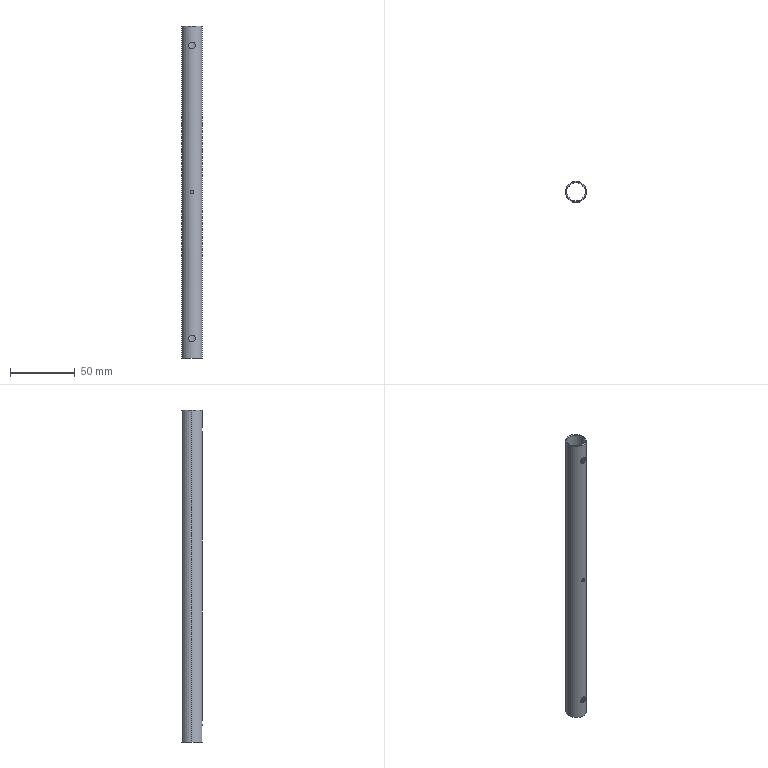Part | SolidWorks | features BaseBody 1 | 1 solid | 12 faces | box 16 x 16 x 256 mm | volume 9739 mm3 | cylinder 10 | plane 2 | commonest cylinder face diameters 5.2 x4 3 x2 14.4 x2 16 x2
STEP:
#1=CARTESIAN_POINT('',(-8.,0.,256.));
#2=VERTEX_POINT('',#1);
#3=CARTESIAN_POINT('',(8.,0.,256.));
#4=VERTEX_POINT('',#3);
#5=CARTESIAN_POINT('',(0.,0.,256.));
#6=DIRECTION('',(0.,0.,-1.));
#7=DIRECTION('',(-1.,0.,0.));
#8=AXIS2_PLACEMENT_3D('',#5,#6,#7);
#9=CIRCLE('',#8,8.);
#10=EDGE_CURVE('',#2,#4,#9,.T.);
#11=ORIENTED_EDGE('',*,*,#10,.T.);
#12=CARTESIAN_POINT('',(8.,0.,0.));
#13=VERTEX_POINT('',#12);
#14=CARTESIAN_POINT('',(8.,0.,256.));
#15=DIRECTION('',(0.,0.,-1.));
#16=VECTOR('',#15,1000.);
#17=LINE('',#14,#16);
#18=EDGE_CURVE('',#4,#13,#17,.T.);
#19=ORIENTED_EDGE('',*,*,#18,.T.);
#20=CARTESIAN_POINT('',(-8.,0.,0.));
#21=VERTEX_POINT('',#20);
#22=CARTESIAN_POINT('',(0.,0.,0.));
#23=DIRECTION('',(0.,0.,1.));
#24=DIRECTION('',(-1.,0.,0.));
#25=AXIS2_PLACEMENT_3D('',#22,#23,#24);
#26=CIRCLE('',#25,8.);
#27=EDGE_CURVE('',#13,#21,#26,.T.);
#28=ORIENTED_EDGE('',*,*,#27,.T.);
#29=CARTESIAN_POINT('',(-8.,0.,256.));
#30=DIRECTION('',(0.,0.,-1.));
#31=VECTOR('',#30,1000.);
#32=LINE('',#29,#31);
#33=EDGE_CURVE('',#2,#21,#32,.T.);
#34=ORIENTED_EDGE('',*,*,#33,.F.);
#35=EDGE_LOOP('',(#11,#19,#28,#34));
#36=FACE_OUTER_BOUND('',#35,.T.);
#37=CARTESIAN_POINT('',(0.,0.,256.));
#38=DIRECTION('',(0.,0.,-1.));
#39=DIRECTION('',(-1.,0.,0.));
#40=AXIS2_PLACEMENT_3D('',#37,#38,#39);
#41=CYLINDRICAL_SURFACE('',#40,8.);
#42=ADVANCED_FACE('',(#36),#41,.T.);
#43=CARTESIAN_POINT('',(0.,-8.,126.5));
#44=VERTEX_POINT('',#43);
#45=CARTESIAN_POINT('',(0.,-8.,129.5));
#46=VERTEX_POINT('',#45);
#47=CARTESIAN_POINT('',(0.,-8.,126.5));
#48=CARTESIAN_POINT('',(-0.09932,-8.,126.5));
#49=CARTESIAN_POINT('',(-0.1969,-7.998,126.51));
#50=CARTESIAN_POINT('',(-0.3889,-7.991,126.548));
#51=CARTESIAN_POINT('',(-0.4843,-7.986,126.577));
#52=CARTESIAN_POINT('',(-0.6658,-7.973,126.652));
#53=CARTESIAN_POINT('',(-0.7519,-7.965,126.698));
#54=CARTESIAN_POINT('',(-0.9148,-7.948,126.807));
#55=CARTESIAN_POINT('',(-0.9917,-7.939,126.87));
#56=CARTESIAN_POINT('',(-1.199,-7.911,127.077));
#57=CARTESIAN_POINT('',(-1.31,-7.892,127.244));
#58=CARTESIAN_POINT('',(-1.46,-7.866,127.605));
#59=CARTESIAN_POINT('',(-1.5,-7.858,127.803));
#60=CARTESIAN_POINT('',(-1.5,-7.858,128.097));
#61=CARTESIAN_POINT('',(-1.49,-7.86,128.196));
#62=CARTESIAN_POINT('',(-1.452,-7.867,128.389));
#63=CARTESIAN_POINT('',(-1.424,-7.872,128.483));
#64=CARTESIAN_POINT('',(-1.311,-7.892,128.755));
#65=CARTESIAN_POINT('',(-1.201,-7.911,128.92));
#66=CARTESIAN_POINT('',(-0.9916,-7.939,129.13));
#67=CARTESIAN_POINT('',(-0.9161,-7.948,129.192));
#68=CARTESIAN_POINT('',(-0.7539,-7.965,129.3));
#69=CARTESIAN_POINT('',(-0.6662,-7.973,129.348));
#70=CARTESIAN_POINT('',(-0.3942,-7.992,129.461));
#71=CARTESIAN_POINT('',(-0.1986,-8.,129.5));
#72=CARTESIAN_POINT('',(0.,-8.,129.5));
#73=B_SPLINE_CURVE_WITH_KNOTS('',3,(#47,#48,#49,#50,#51,#52,#53,#54,#55,#56,#57,#58,#59,#60,#61,#62,#63,#64,#65,#66,#67,#68,#69,#70,#71,#72),.UNSPECIFIED.,.F.,.F.,(4,2,2,2,2,2,2,2,2,2,2,2,4),(0.,0.0002937,0.0005874,0.000881,0.001175,0.001762,0.002349,0.002643,0.002937,0.003524,0.003818,0.004112,0.004699),.UNSPECIFIED.);
#74=EDGE_CURVE('',#44,#46,#73,.T.);
#75=ORIENTED_EDGE('',*,*,#74,.F.);
#76=CARTESIAN_POINT('',(0.,-7.2,126.5));
#77=VERTEX_POINT('',#76);
#78=CARTESIAN_POINT('',(0.,-8.,126.5));
#79=DIRECTION('',(0.,1.,0.));
#80=VECTOR('',#79,1000.);
#81=LINE('',#78,#80);
#82=EDGE_CURVE('',#44,#77,#81,.T.);
#83=ORIENTED_EDGE('',*,*,#82,.T.);
#84=CARTESIAN_POINT('',(0.,-7.2,129.5));
#85=VERTEX_POINT('',#84);
#86=CARTESIAN_POINT('',(0.,-7.2,129.5));
#87=CARTESIAN_POINT('',(-0.09937,-7.2,129.5));
#88=CARTESIAN_POINT('',(-0.197,-7.198,129.49));
#89=CARTESIAN_POINT('',(-0.3891,-7.19,129.452));
#90=CARTESIAN_POINT('',(-0.4845,-7.184,129.423));
#91=CARTESIAN_POINT('',(-0.666,-7.17,129.348));
#92=CARTESIAN_POINT('',(-0.752,-7.161,129.302));
#93=CARTESIAN_POINT('',(-0.9149,-7.142,129.193));
#94=CARTESIAN_POINT('',(-0.9917,-7.132,129.13));
#95=CARTESIAN_POINT('',(-1.199,-7.101,128.923));
#96=CARTESIAN_POINT('',(-1.31,-7.08,128.756));
#97=CARTESIAN_POINT('',(-1.46,-7.051,128.395));
#98=CARTESIAN_POINT('',(-1.5,-7.042,128.197));
#99=CARTESIAN_POINT('',(-1.5,-7.042,127.903));
#100=CARTESIAN_POINT('',(-1.49,-7.044,127.803));
#101=CARTESIAN_POINT('',(-1.452,-7.052,127.611));
#102=CARTESIAN_POINT('',(-1.424,-7.058,127.517));
#103=CARTESIAN_POINT('',(-1.311,-7.08,127.244));
#104=CARTESIAN_POINT('',(-1.2,-7.101,127.079));
#105=CARTESIAN_POINT('',(-0.9916,-7.132,126.87));
#106=CARTESIAN_POINT('',(-0.9162,-7.142,126.808));
#107=CARTESIAN_POINT('',(-0.7541,-7.161,126.7));
#108=CARTESIAN_POINT('',(-0.6663,-7.17,126.653));
#109=CARTESIAN_POINT('',(-0.3945,-7.191,126.54));
#110=CARTESIAN_POINT('',(-0.1988,-7.2,126.5));
#111=CARTESIAN_POINT('',(0.,-7.2,126.5));
#112=B_SPLINE_CURVE_WITH_KNOTS('',3,(#86,#87,#88,#89,#90,#91,#92,#93,#94,#95,#96,#97,#98,#99,#100,#101,#102,#103,#104,#105,#106,#107,#108,#109,#110,#111),.UNSPECIFIED.,.F.,.F.,(4,2,2,2,2,2,2,2,2,2,2,2,4),(0.,0.0002938,0.0005877,0.0008815,0.001175,0.001763,0.002351,0.002644,0.002938,0.003526,0.00382,0.004114,0.004701),.UNSPECIFIED.);
#113=EDGE_CURVE('',#85,#77,#112,.T.);
#114=ORIENTED_EDGE('',*,*,#113,.F.);
#115=CARTESIAN_POINT('',(0.,-8.,129.5));
#116=DIRECTION('',(0.,1.,0.));
#117=VECTOR('',#116,1000.);
#118=LINE('',#115,#117);
#119=EDGE_CURVE('',#46,#85,#118,.T.);
#120=ORIENTED_EDGE('',*,*,#119,.F.);
#121=EDGE_LOOP('',(#75,#83,#114,#120));
#122=FACE_OUTER_BOUND('',#121,.T.);
#123=CARTESIAN_POINT('',(0.,-8.,128.));
#124=DIRECTION('',(0.,1.,0.));
#125=DIRECTION('',(0.,0.,1.));
#126=AXIS2_PLACEMENT_3D('',#123,#124,#125);
#127=CYLINDRICAL_SURFACE('',#126,1.5);
#128=ADVANCED_FACE('',(#122),#127,.F.);
#129=CARTESIAN_POINT('',(0.,-8.,238.4));
#130=VERTEX_POINT('',#129);
#131=CARTESIAN_POINT('',(0.,-8.,243.6));
#132=VERTEX_POINT('',#131);
#133=CARTESIAN_POINT('',(0.,-8.,238.4));
#134=CARTESIAN_POINT('',(-0.173,-8.,238.4));
#135=CARTESIAN_POINT('',(-0.3429,-7.994,238.417));
#136=CARTESIAN_POINT('',(-0.6767,-7.973,238.484));
#137=CARTESIAN_POINT('',(-0.8425,-7.957,238.534));
#138=CARTESIAN_POINT('',(-1.157,-7.918,238.665));
#139=CARTESIAN_POINT('',(-1.306,-7.894,238.745));
#140=CARTESIAN_POINT('',(-1.587,-7.842,238.934));
#141=CARTESIAN_POINT('',(-1.72,-7.814,239.043));
#142=CARTESIAN_POINT('',(-2.077,-7.73,239.4));
#143=CARTESIAN_POINT('',(-2.27,-7.672,239.688));
#144=CARTESIAN_POINT('',(-2.465,-7.611,240.156));
#145=CARTESIAN_POINT('',(-2.516,-7.594,240.321));
#146=CARTESIAN_POINT('',(-2.583,-7.572,240.657));
#147=CARTESIAN_POINT('',(-2.6,-7.566,240.826));
#148=CARTESIAN_POINT('',(-2.6,-7.566,241.168));
#149=CARTESIAN_POINT('',(-2.583,-7.572,241.342));
#150=CARTESIAN_POINT('',(-2.516,-7.594,241.676));
#151=CARTESIAN_POINT('',(-2.467,-7.61,241.839));
#152=CARTESIAN_POINT('',(-2.336,-7.652,242.155));
#153=CARTESIAN_POINT('',(-2.255,-7.676,242.305));
#154=CARTESIAN_POINT('',(-2.068,-7.729,242.585));
#155=CARTESIAN_POINT('',(-1.959,-7.757,242.718));
#156=CARTESIAN_POINT('',(-1.72,-7.814,242.957));
#157=CARTESIAN_POINT('',(-1.59,-7.842,243.064));
#158=CARTESIAN_POINT('',(-1.309,-7.893,243.253));
#159=CARTESIAN_POINT('',(-1.157,-7.917,243.334));
#160=CARTESIAN_POINT('',(-0.8442,-7.957,243.465));
#161=CARTESIAN_POINT('',(-0.682,-7.973,243.515));
#162=CARTESIAN_POINT('',(-0.3459,-7.994,243.583));
#163=CARTESIAN_POINT('',(-0.173,-8.,243.6));
#164=CARTESIAN_POINT('',(0.,-8.,243.6));
#165=B_SPLINE_CURVE_WITH_KNOTS('',3,(#133,#134,#135,#136,#137,#138,#139,#140,#141,#142,#143,#144,#145,#146,#147,#148,#149,#150,#151,#152,#153,#154,#155,#156,#157,#158,#159,#160,#161,#162,#163,#164),.UNSPECIFIED.,.F.,.F.,(4,2,2,2,2,2,2,2,2,2,2,2,2,2,2,4),(0.,0.0005114,0.001023,0.001534,0.002045,0.003068,0.003579,0.004091,0.004602,0.005114,0.005625,0.006136,0.006648,0.007159,0.00767,0.008182),.UNSPECIFIED.);
#166=EDGE_CURVE('',#130,#132,#165,.T.);
#167=ORIENTED_EDGE('',*,*,#166,.F.);
#168=CARTESIAN_POINT('',(0.,-7.2,238.4));
#169=VERTEX_POINT('',#168);
#170=CARTESIAN_POINT('',(0.,-8.,238.4));
#171=DIRECTION('',(0.,1.,0.));
#172=VECTOR('',#171,1000.);
#173=LINE('',#170,#172);
#174=EDGE_CURVE('',#130,#169,#173,.T.);
#175=ORIENTED_EDGE('',*,*,#174,.T.);
#176=CARTESIAN_POINT('',(0.,-7.2,243.6));
#177=VERTEX_POINT('',#176);
#178=CARTESIAN_POINT('',(0.,-7.2,243.6));
#179=CARTESIAN_POINT('',(-0.1733,-7.2,243.6));
#180=CARTESIAN_POINT('',(-0.3434,-7.194,243.583));
#181=CARTESIAN_POINT('',(-0.6777,-7.17,243.516));
#182=CARTESIAN_POINT('',(-0.8436,-7.152,243.465));
#183=CARTESIAN_POINT('',(-1.158,-7.108,243.334));
#184=CARTESIAN_POINT('',(-1.307,-7.082,243.254));
#185=CARTESIAN_POINT('',(-1.588,-7.024,243.066));
#186=CARTESIAN_POINT('',(-1.72,-6.993,242.957));
#187=CARTESIAN_POINT('',(-2.076,-6.898,242.6));
#188=CARTESIAN_POINT('',(-2.269,-6.834,242.313));
#189=CARTESIAN_POINT('',(-2.465,-6.765,241.845));
#190=CARTESIAN_POINT('',(-2.515,-6.746,241.68));
#191=CARTESIAN_POINT('',(-2.583,-6.721,241.344));
#192=CARTESIAN_POINT('',(-2.6,-6.714,241.174));
#193=CARTESIAN_POINT('',(-2.6,-6.714,240.832));
#194=CARTESIAN_POINT('',(-2.583,-6.721,240.658));
#195=CARTESIAN_POINT('',(-2.516,-6.746,240.323));
#196=CARTESIAN_POINT('',(-2.467,-6.765,240.161));
#197=CARTESIAN_POINT('',(-2.335,-6.811,239.844));
#198=CARTESIAN_POINT('',(-2.255,-6.839,239.694));
#199=CARTESIAN_POINT('',(-2.067,-6.898,239.414));
#200=CARTESIAN_POINT('',(-1.959,-6.93,239.282));
#201=CARTESIAN_POINT('',(-1.72,-6.993,239.043));
#202=CARTESIAN_POINT('',(-1.591,-7.024,238.936));
#203=CARTESIAN_POINT('',(-1.31,-7.081,238.748));
#204=CARTESIAN_POINT('',(-1.158,-7.108,238.666));
#205=CARTESIAN_POINT('',(-0.8456,-7.152,238.536));
#206=CARTESIAN_POINT('',(-0.6833,-7.169,238.486));
#207=CARTESIAN_POINT('',(-0.3462,-7.194,238.417));
#208=CARTESIAN_POINT('',(-0.1733,-7.2,238.4));
#209=CARTESIAN_POINT('',(0.,-7.2,238.4));
#210=B_SPLINE_CURVE_WITH_KNOTS('',3,(#178,#179,#180,#181,#182,#183,#184,#185,#186,#187,#188,#189,#190,#191,#192,#193,#194,#195,#196,#197,#198,#199,#200,#201,#202,#203,#204,#205,#206,#207,#208,#209),.UNSPECIFIED.,.F.,.F.,(4,2,2,2,2,2,2,2,2,2,2,2,2,2,2,4),(0.,0.0005122,0.001024,0.001537,0.002049,0.003073,0.003585,0.004098,0.00461,0.005122,0.005634,0.006146,0.006659,0.007171,0.007683,0.008195),.UNSPECIFIED.);
#211=EDGE_CURVE('',#177,#169,#210,.T.);
#212=ORIENTED_EDGE('',*,*,#211,.F.);
#213=CARTESIAN_POINT('',(0.,-8.,243.6));
#214=DIRECTION('',(0.,1.,0.));
#215=VECTOR('',#214,1000.);
#216=LINE('',#213,#215);
#217=EDGE_CURVE('',#132,#177,#216,.T.);
#218=ORIENTED_EDGE('',*,*,#217,.F.);
#219=EDGE_LOOP('',(#167,#175,#212,#218));
#220=FACE_OUTER_BOUND('',#219,.T.);
#221=CARTESIAN_POINT('',(0.,-8.,241.));
#222=DIRECTION('',(0.,1.,0.));
#223=DIRECTION('',(0.,0.,1.));
#224=AXIS2_PLACEMENT_3D('',#221,#222,#223);
#225=CYLINDRICAL_SURFACE('',#224,2.6);
#226=ADVANCED_FACE('',(#220),#225,.F.);
#227=CARTESIAN_POINT('',(0.,-8.,12.4));
#228=VERTEX_POINT('',#227);
#229=CARTESIAN_POINT('',(0.,-8.,17.6));
#230=VERTEX_POINT('',#229);
#231=CARTESIAN_POINT('',(0.,-8.,12.4));
#232=CARTESIAN_POINT('',(-0.173,-8.,12.4));
#233=CARTESIAN_POINT('',(-0.3429,-7.994,12.417));
#234=CARTESIAN_POINT('',(-0.6767,-7.973,12.484));
#235=CARTESIAN_POINT('',(-0.8425,-7.957,12.534));
#236=CARTESIAN_POINT('',(-1.157,-7.918,12.665));
#237=CARTESIAN_POINT('',(-1.306,-7.894,12.745));
#238=CARTESIAN_POINT('',(-1.587,-7.842,12.934));
#239=CARTESIAN_POINT('',(-1.72,-7.814,13.043));
#240=CARTESIAN_POINT('',(-2.077,-7.73,13.4));
#241=CARTESIAN_POINT('',(-2.27,-7.672,13.688));
#242=CARTESIAN_POINT('',(-2.465,-7.611,14.156));
#243=CARTESIAN_POINT('',(-2.516,-7.594,14.321));
#244=CARTESIAN_POINT('',(-2.583,-7.572,14.657));
#245=CARTESIAN_POINT('',(-2.6,-7.566,14.826));
#246=CARTESIAN_POINT('',(-2.6,-7.566,15.168));
#247=CARTESIAN_POINT('',(-2.583,-7.572,15.342));
#248=CARTESIAN_POINT('',(-2.516,-7.594,15.676));
#249=CARTESIAN_POINT('',(-2.467,-7.61,15.839));
#250=CARTESIAN_POINT('',(-2.336,-7.652,16.155));
#251=CARTESIAN_POINT('',(-2.255,-7.676,16.305));
#252=CARTESIAN_POINT('',(-2.068,-7.729,16.585));
#253=CARTESIAN_POINT('',(-1.959,-7.757,16.718));
#254=CARTESIAN_POINT('',(-1.72,-7.814,16.957));
#255=CARTESIAN_POINT('',(-1.59,-7.842,17.064));
#256=CARTESIAN_POINT('',(-1.309,-7.893,17.253));
#257=CARTESIAN_POINT('',(-1.157,-7.917,17.334));
#258=CARTESIAN_POINT('',(-0.8442,-7.957,17.465));
#259=CARTESIAN_POINT('',(-0.682,-7.973,17.515));
#260=CARTESIAN_POINT('',(-0.3459,-7.994,17.583));
#261=CARTESIAN_POINT('',(-0.173,-8.,17.6));
#262=CARTESIAN_POINT('',(0.,-8.,17.6));
#263=B_SPLINE_CURVE_WITH_KNOTS('',3,(#231,#232,#233,#234,#235,#236,#237,#238,#239,#240,#241,#242,#243,#244,#245,#246,#247,#248,#249,#250,#251,#252,#253,#254,#255,#256,#257,#258,#259,#260,#261,#262),.UNSPECIFIED.,.F.,.F.,(4,2,2,2,2,2,2,2,2,2,2,2,2,2,2,4),(0.,0.0005114,0.001023,0.001534,0.002045,0.003068,0.003579,0.004091,0.004602,0.005114,0.005625,0.006136,0.006648,0.007159,0.00767,0.008182),.UNSPECIFIED.);
#264=EDGE_CURVE('',#228,#230,#263,.T.);
#265=ORIENTED_EDGE('',*,*,#264,.F.);
#266=CARTESIAN_POINT('',(0.,-7.2,12.4));
#267=VERTEX_POINT('',#266);
#268=CARTESIAN_POINT('',(0.,-8.,12.4));
#269=DIRECTION('',(0.,1.,0.));
#270=VECTOR('',#269,1000.);
#271=LINE('',#268,#270);
#272=EDGE_CURVE('',#228,#267,#271,.T.);
#273=ORIENTED_EDGE('',*,*,#272,.T.);
#274=CARTESIAN_POINT('',(0.,-7.2,17.6));
#275=VERTEX_POINT('',#274);
#276=CARTESIAN_POINT('',(0.,-7.2,17.6));
#277=CARTESIAN_POINT('',(-0.1733,-7.2,17.6));
#278=CARTESIAN_POINT('',(-0.3434,-7.194,17.583));
#279=CARTESIAN_POINT('',(-0.6777,-7.17,17.516));
#280=CARTESIAN_POINT('',(-0.8436,-7.152,17.465));
#281=CARTESIAN_POINT('',(-1.158,-7.108,17.334));
#282=CARTESIAN_POINT('',(-1.307,-7.082,17.254));
#283=CARTESIAN_POINT('',(-1.588,-7.024,17.066));
#284=CARTESIAN_POINT('',(-1.72,-6.993,16.957));
#285=CARTESIAN_POINT('',(-2.076,-6.898,16.6));
#286=CARTESIAN_POINT('',(-2.269,-6.834,16.313));
#287=CARTESIAN_POINT('',(-2.465,-6.765,15.845));
#288=CARTESIAN_POINT('',(-2.515,-6.746,15.68));
#289=CARTESIAN_POINT('',(-2.583,-6.721,15.344));
#290=CARTESIAN_POINT('',(-2.6,-6.714,15.174));
#291=CARTESIAN_POINT('',(-2.6,-6.714,14.832));
#292=CARTESIAN_POINT('',(-2.583,-6.721,14.658));
#293=CARTESIAN_POINT('',(-2.516,-6.746,14.323));
#294=CARTESIAN_POINT('',(-2.467,-6.765,14.161));
#295=CARTESIAN_POINT('',(-2.335,-6.811,13.844));
#296=CARTESIAN_POINT('',(-2.255,-6.839,13.694));
#297=CARTESIAN_POINT('',(-2.067,-6.898,13.414));
#298=CARTESIAN_POINT('',(-1.959,-6.93,13.282));
#299=CARTESIAN_POINT('',(-1.72,-6.993,13.043));
#300=CARTESIAN_POINT('',(-1.591,-7.024,12.936));
#301=CARTESIAN_POINT('',(-1.31,-7.081,12.748));
#302=CARTESIAN_POINT('',(-1.158,-7.108,12.666));
#303=CARTESIAN_POINT('',(-0.8456,-7.152,12.536));
#304=CARTESIAN_POINT('',(-0.6833,-7.169,12.486));
#305=CARTESIAN_POINT('',(-0.3462,-7.194,12.417));
#306=CARTESIAN_POINT('',(-0.1733,-7.2,12.4));
#307=CARTESIAN_POINT('',(0.,-7.2,12.4));
#308=B_SPLINE_CURVE_WITH_KNOTS('',3,(#276,#277,#278,#279,#280,#281,#282,#283,#284,#285,#286,#287,#288,#289,#290,#291,#292,#293,#294,#295,#296,#297,#298,#299,#300,#301,#302,#303,#304,#305,#306,#307),.UNSPECIFIED.,.F.,.F.,(4,2,2,2,2,2,2,2,2,2,2,2,2,2,2,4),(0.,0.0005122,0.001024,0.001537,0.002049,0.003073,0.003585,0.004098,0.00461,0.005122,0.005634,0.006146,0.006659,0.007171,0.007683,0.008195),.UNSPECIFIED.);
#309=EDGE_CURVE('',#275,#267,#308,.T.);
#310=ORIENTED_EDGE('',*,*,#309,.F.);
#311=CARTESIAN_POINT('',(0.,-8.,17.6));
#312=DIRECTION('',(0.,1.,0.));
#313=VECTOR('',#312,1000.);
#314=LINE('',#311,#313);
#315=EDGE_CURVE('',#230,#275,#314,.T.);
#316=ORIENTED_EDGE('',*,*,#315,.F.);
#317=EDGE_LOOP('',(#265,#273,#310,#316));
#318=FACE_OUTER_BOUND('',#317,.T.);
#319=CARTESIAN_POINT('',(0.,-8.,15.));
#320=DIRECTION('',(0.,1.,0.));
#321=DIRECTION('',(0.,0.,1.));
#322=AXIS2_PLACEMENT_3D('',#319,#320,#321);
#323=CYLINDRICAL_SURFACE('',#322,2.6);
#324=ADVANCED_FACE('',(#318),#323,.F.);
#325=ORIENTED_EDGE('',*,*,#113,.T.);
#326=CARTESIAN_POINT('',(0.,-7.2,126.5));
#327=CARTESIAN_POINT('',(0.09937,-7.2,126.5));
#328=CARTESIAN_POINT('',(0.197,-7.198,126.51));
#329=CARTESIAN_POINT('',(0.3891,-7.19,126.548));
#330=CARTESIAN_POINT('',(0.4845,-7.184,126.577));
#331=CARTESIAN_POINT('',(0.666,-7.17,126.652));
#332=CARTESIAN_POINT('',(0.752,-7.161,126.698));
#333=CARTESIAN_POINT('',(0.9149,-7.142,126.807));
#334=CARTESIAN_POINT('',(0.9917,-7.132,126.87));
#335=CARTESIAN_POINT('',(1.199,-7.101,127.077));
#336=CARTESIAN_POINT('',(1.31,-7.08,127.244));
#337=CARTESIAN_POINT('',(1.46,-7.051,127.605));
#338=CARTESIAN_POINT('',(1.5,-7.042,127.803));
#339=CARTESIAN_POINT('',(1.5,-7.042,128.097));
#340=CARTESIAN_POINT('',(1.49,-7.044,128.197));
#341=CARTESIAN_POINT('',(1.452,-7.052,128.389));
#342=CARTESIAN_POINT('',(1.424,-7.058,128.483));
#343=CARTESIAN_POINT('',(1.311,-7.08,128.756));
#344=CARTESIAN_POINT('',(1.2,-7.101,128.921));
#345=CARTESIAN_POINT('',(0.9916,-7.132,129.13));
#346=CARTESIAN_POINT('',(0.9162,-7.142,129.192));
#347=CARTESIAN_POINT('',(0.7541,-7.161,129.3));
#348=CARTESIAN_POINT('',(0.6663,-7.17,129.347));
#349=CARTESIAN_POINT('',(0.3945,-7.191,129.46));
#350=CARTESIAN_POINT('',(0.1987,-7.2,129.5));
#351=CARTESIAN_POINT('',(0.,-7.2,129.5));
#352=B_SPLINE_CURVE_WITH_KNOTS('',3,(#326,#327,#328,#329,#330,#331,#332,#333,#334,#335,#336,#337,#338,#339,#340,#341,#342,#343,#344,#345,#346,#347,#348,#349,#350,#351),.UNSPECIFIED.,.F.,.F.,(4,2,2,2,2,2,2,2,2,2,2,2,4),(0.004701,0.004995,0.005289,0.005583,0.005877,0.006464,0.007052,0.007346,0.00764,0.008227,0.008521,0.008815,0.009403),.UNSPECIFIED.);
#353=EDGE_CURVE('',#77,#85,#352,.T.);
#354=ORIENTED_EDGE('',*,*,#353,.T.);
#355=EDGE_LOOP('',(#325,#354));
#356=FACE_BOUND('',#355,.T.);
#357=ORIENTED_EDGE('',*,*,#211,.T.);
#358=CARTESIAN_POINT('',(0.,-7.2,238.4));
#359=CARTESIAN_POINT('',(0.1733,-7.2,238.4));
#360=CARTESIAN_POINT('',(0.3434,-7.194,238.417));
#361=CARTESIAN_POINT('',(0.6777,-7.17,238.484));
#362=CARTESIAN_POINT('',(0.8436,-7.152,238.535));
#363=CARTESIAN_POINT('',(1.158,-7.108,238.666));
#364=CARTESIAN_POINT('',(1.307,-7.082,238.746));
#365=CARTESIAN_POINT('',(1.588,-7.024,238.934));
#366=CARTESIAN_POINT('',(1.72,-6.993,239.043));
#367=CARTESIAN_POINT('',(2.076,-6.898,239.4));
#368=CARTESIAN_POINT('',(2.269,-6.834,239.687));
#369=CARTESIAN_POINT('',(2.465,-6.765,240.155));
#370=CARTESIAN_POINT('',(2.515,-6.746,240.32));
#371=CARTESIAN_POINT('',(2.583,-6.721,240.656));
#372=CARTESIAN_POINT('',(2.6,-6.714,240.826));
#373=CARTESIAN_POINT('',(2.6,-6.714,241.168));
#374=CARTESIAN_POINT('',(2.583,-6.721,241.342));
#375=CARTESIAN_POINT('',(2.516,-6.746,241.677));
#376=CARTESIAN_POINT('',(2.467,-6.765,241.839));
#377=CARTESIAN_POINT('',(2.335,-6.811,242.156));
#378=CARTESIAN_POINT('',(2.255,-6.839,242.306));
#379=CARTESIAN_POINT('',(2.067,-6.898,242.586));
#380=CARTESIAN_POINT('',(1.959,-6.93,242.718));
#381=CARTESIAN_POINT('',(1.72,-6.993,242.957));
#382=CARTESIAN_POINT('',(1.591,-7.024,243.064));
#383=CARTESIAN_POINT('',(1.31,-7.081,243.252));
#384=CARTESIAN_POINT('',(1.158,-7.108,243.334));
#385=CARTESIAN_POINT('',(0.8456,-7.152,243.464));
#386=CARTESIAN_POINT('',(0.6833,-7.169,243.514));
#387=CARTESIAN_POINT('',(0.3462,-7.194,243.583));
#388=CARTESIAN_POINT('',(0.1733,-7.2,243.6));
#389=CARTESIAN_POINT('',(0.,-7.2,243.6));
#390=B_SPLINE_CURVE_WITH_KNOTS('',3,(#358,#359,#360,#361,#362,#363,#364,#365,#366,#367,#368,#369,#370,#371,#372,#373,#374,#375,#376,#377,#378,#379,#380,#381,#382,#383,#384,#385,#386,#387,#388,#389),.UNSPECIFIED.,.F.,.F.,(4,2,2,2,2,2,2,2,2,2,2,2,2,2,2,4),(0.008195,0.008707,0.00922,0.009732,0.01024,0.01127,0.01178,0.01229,0.0128,0.01332,0.01383,0.01434,0.01485,0.01536,0.01588,0.01639),.UNSPECIFIED.);
#391=EDGE_CURVE('',#169,#177,#390,.T.);
#392=ORIENTED_EDGE('',*,*,#391,.T.);
#393=EDGE_LOOP('',(#357,#392));
#394=FACE_BOUND('',#393,.T.);
#395=ORIENTED_EDGE('',*,*,#309,.T.);
#396=CARTESIAN_POINT('',(0.,-7.2,12.4));
#397=CARTESIAN_POINT('',(0.1733,-7.2,12.4));
#398=CARTESIAN_POINT('',(0.3434,-7.194,12.417));
#399=CARTESIAN_POINT('',(0.6777,-7.17,12.484));
#400=CARTESIAN_POINT('',(0.8436,-7.152,12.535));
#401=CARTESIAN_POINT('',(1.158,-7.108,12.666));
#402=CARTESIAN_POINT('',(1.307,-7.082,12.746));
#403=CARTESIAN_POINT('',(1.588,-7.024,12.934));
#404=CARTESIAN_POINT('',(1.72,-6.993,13.043));
#405=CARTESIAN_POINT('',(2.076,-6.898,13.4));
#406=CARTESIAN_POINT('',(2.269,-6.834,13.687));
#407=CARTESIAN_POINT('',(2.465,-6.765,14.155));
#408=CARTESIAN_POINT('',(2.515,-6.746,14.32));
#409=CARTESIAN_POINT('',(2.583,-6.721,14.656));
#410=CARTESIAN_POINT('',(2.6,-6.714,14.826));
#411=CARTESIAN_POINT('',(2.6,-6.714,15.168));
#412=CARTESIAN_POINT('',(2.583,-6.721,15.342));
#413=CARTESIAN_POINT('',(2.516,-6.746,15.677));
#414=CARTESIAN_POINT('',(2.467,-6.765,15.839));
#415=CARTESIAN_POINT('',(2.335,-6.811,16.156));
#416=CARTESIAN_POINT('',(2.255,-6.839,16.306));
#417=CARTESIAN_POINT('',(2.067,-6.898,16.586));
#418=CARTESIAN_POINT('',(1.959,-6.93,16.718));
#419=CARTESIAN_POINT('',(1.72,-6.993,16.957));
#420=CARTESIAN_POINT('',(1.591,-7.024,17.064));
#421=CARTESIAN_POINT('',(1.31,-7.081,17.252));
#422=CARTESIAN_POINT('',(1.158,-7.108,17.334));
#423=CARTESIAN_POINT('',(0.8456,-7.152,17.464));
#424=CARTESIAN_POINT('',(0.6833,-7.169,17.514));
#425=CARTESIAN_POINT('',(0.3462,-7.194,17.583));
#426=CARTESIAN_POINT('',(0.1733,-7.2,17.6));
#427=CARTESIAN_POINT('',(0.,-7.2,17.6));
#428=B_SPLINE_CURVE_WITH_KNOTS('',3,(#396,#397,#398,#399,#400,#401,#402,#403,#404,#405,#406,#407,#408,#409,#410,#411,#412,#413,#414,#415,#416,#417,#418,#419,#420,#421,#422,#423,#424,#425,#426,#427),.UNSPECIFIED.,.F.,.F.,(4,2,2,2,2,2,2,2,2,2,2,2,2,2,2,4),(0.008195,0.008707,0.00922,0.009732,0.01024,0.01127,0.01178,0.01229,0.0128,0.01332,0.01383,0.01434,0.01485,0.01536,0.01588,0.01639),.UNSPECIFIED.);
#429=EDGE_CURVE('',#267,#275,#428,.T.);
#430=ORIENTED_EDGE('',*,*,#429,.T.);
#431=EDGE_LOOP('',(#395,#430));
#432=FACE_BOUND('',#431,.T.);
#433=CARTESIAN_POINT('',(7.2,0.,256.));
#434=VERTEX_POINT('',#433);
#435=CARTESIAN_POINT('',(-7.2,0.,256.));
#436=VERTEX_POINT('',#435);
#437=CARTESIAN_POINT('',(0.,0.,256.));
#438=DIRECTION('',(0.,0.,-1.));
#439=DIRECTION('',(-1.,0.,0.));
#440=AXIS2_PLACEMENT_3D('',#437,#438,#439);
#441=CIRCLE('',#440,7.2);
#442=EDGE_CURVE('',#434,#436,#441,.T.);
#443=ORIENTED_EDGE('',*,*,#442,.F.);
#444=CARTESIAN_POINT('',(7.2,0.,0.));
#445=VERTEX_POINT('',#444);
#446=CARTESIAN_POINT('',(7.2,0.,256.));
#447=DIRECTION('',(0.,0.,-1.));
#448=VECTOR('',#447,1000.);
#449=LINE('',#446,#448);
#450=EDGE_CURVE('',#434,#445,#449,.T.);
#451=ORIENTED_EDGE('',*,*,#450,.T.);
#452=CARTESIAN_POINT('',(-7.2,0.,0.));
#453=VERTEX_POINT('',#452);
#454=CARTESIAN_POINT('',(0.,0.,0.));
#455=DIRECTION('',(0.,0.,-1.));
#456=DIRECTION('',(-1.,0.,0.));
#457=AXIS2_PLACEMENT_3D('',#454,#455,#456);
#458=CIRCLE('',#457,7.2);
#459=EDGE_CURVE('',#445,#453,#458,.T.);
#460=ORIENTED_EDGE('',*,*,#459,.T.);
#461=CARTESIAN_POINT('',(-7.2,0.,256.));
#462=DIRECTION('',(0.,0.,-1.));
#463=VECTOR('',#462,1000.);
#464=LINE('',#461,#463);
#465=EDGE_CURVE('',#436,#453,#464,.T.);
#466=ORIENTED_EDGE('',*,*,#465,.F.);
#467=EDGE_LOOP('',(#443,#451,#460,#466));
#468=FACE_OUTER_BOUND('',#467,.T.);
#469=CARTESIAN_POINT('',(0.,0.,256.));
#470=DIRECTION('',(0.,0.,-1.));
#471=DIRECTION('',(-1.,0.,0.));
#472=AXIS2_PLACEMENT_3D('',#469,#470,#471);
#473=CYLINDRICAL_SURFACE('',#472,7.2);
#474=ADVANCED_FACE('',(#356,#394,#432,#468),#473,.F.);
#475=ORIENTED_EDGE('',*,*,#18,.F.);
#476=CARTESIAN_POINT('',(0.,0.,256.));
#477=DIRECTION('',(0.,0.,-1.));
#478=DIRECTION('',(-1.,0.,0.));
#479=AXIS2_PLACEMENT_3D('',#476,#477,#478);
#480=CIRCLE('',#479,8.);
#481=EDGE_CURVE('',#4,#2,#480,.T.);
#482=ORIENTED_EDGE('',*,*,#481,.T.);
#483=ORIENTED_EDGE('',*,*,#33,.T.);
#484=CARTESIAN_POINT('',(0.,0.,0.));
#485=DIRECTION('',(0.,0.,1.));
#486=DIRECTION('',(-1.,0.,0.));
#487=AXIS2_PLACEMENT_3D('',#484,#485,#486);
#488=CIRCLE('',#487,8.);
#489=EDGE_CURVE('',#21,#13,#488,.T.);
#490=ORIENTED_EDGE('',*,*,#489,.T.);
#491=EDGE_LOOP('',(#475,#482,#483,#490));
#492=FACE_OUTER_BOUND('',#491,.T.);
#493=CARTESIAN_POINT('',(0.,-8.,129.5));
#494=CARTESIAN_POINT('',(0.09932,-8.,129.5));
#495=CARTESIAN_POINT('',(0.1969,-7.998,129.49));
#496=CARTESIAN_POINT('',(0.3889,-7.991,129.452));
#497=CARTESIAN_POINT('',(0.4843,-7.986,129.423));
#498=CARTESIAN_POINT('',(0.6658,-7.973,129.348));
#499=CARTESIAN_POINT('',(0.7519,-7.965,129.302));
#500=CARTESIAN_POINT('',(0.9148,-7.948,129.193));
#501=CARTESIAN_POINT('',(0.9917,-7.939,129.13));
#502=CARTESIAN_POINT('',(1.199,-7.911,128.923));
#503=CARTESIAN_POINT('',(1.31,-7.892,128.756));
#504=CARTESIAN_POINT('',(1.46,-7.866,128.395));
#505=CARTESIAN_POINT('',(1.5,-7.858,128.197));
#506=CARTESIAN_POINT('',(1.5,-7.858,127.903));
#507=CARTESIAN_POINT('',(1.49,-7.86,127.804));
#508=CARTESIAN_POINT('',(1.452,-7.867,127.611));
#509=CARTESIAN_POINT('',(1.424,-7.872,127.517));
#510=CARTESIAN_POINT('',(1.311,-7.892,127.245));
#511=CARTESIAN_POINT('',(1.201,-7.911,127.08));
#512=CARTESIAN_POINT('',(0.9916,-7.939,126.87));
#513=CARTESIAN_POINT('',(0.9161,-7.948,126.808));
#514=CARTESIAN_POINT('',(0.7539,-7.965,126.7));
#515=CARTESIAN_POINT('',(0.6662,-7.973,126.652));
#516=CARTESIAN_POINT('',(0.3942,-7.992,126.539));
#517=CARTESIAN_POINT('',(0.1986,-8.,126.5));
#518=CARTESIAN_POINT('',(0.,-8.,126.5));
#519=B_SPLINE_CURVE_WITH_KNOTS('',3,(#493,#494,#495,#496,#497,#498,#499,#500,#501,#502,#503,#504,#505,#506,#507,#508,#509,#510,#511,#512,#513,#514,#515,#516,#517,#518),.UNSPECIFIED.,.F.,.F.,(4,2,2,2,2,2,2,2,2,2,2,2,4),(0.004699,0.004993,0.005286,0.00558,0.005874,0.006461,0.007048,0.007342,0.007636,0.008223,0.008517,0.00881,0.009398),.UNSPECIFIED.);
#520=EDGE_CURVE('',#46,#44,#519,.T.);
#521=ORIENTED_EDGE('',*,*,#520,.T.);
#522=ORIENTED_EDGE('',*,*,#74,.T.);
#523=EDGE_LOOP('',(#521,#522));
#524=FACE_BOUND('',#523,.T.);
#525=CARTESIAN_POINT('',(0.,-8.,243.6));
#526=CARTESIAN_POINT('',(0.173,-8.,243.6));
#527=CARTESIAN_POINT('',(0.3429,-7.994,243.583));
#528=CARTESIAN_POINT('',(0.6767,-7.973,243.516));
#529=CARTESIAN_POINT('',(0.8425,-7.957,243.466));
#530=CARTESIAN_POINT('',(1.157,-7.918,243.335));
#531=CARTESIAN_POINT('',(1.306,-7.894,243.255));
#532=CARTESIAN_POINT('',(1.587,-7.842,243.066));
#533=CARTESIAN_POINT('',(1.72,-7.814,242.957));
#534=CARTESIAN_POINT('',(2.077,-7.73,242.6));
#535=CARTESIAN_POINT('',(2.27,-7.672,242.312));
#536=CARTESIAN_POINT('',(2.465,-7.611,241.844));
#537=CARTESIAN_POINT('',(2.516,-7.594,241.679));
#538=CARTESIAN_POINT('',(2.583,-7.572,241.343));
#539=CARTESIAN_POINT('',(2.6,-7.566,241.174));
#540=CARTESIAN_POINT('',(2.6,-7.566,240.832));
#541=CARTESIAN_POINT('',(2.583,-7.572,240.658));
#542=CARTESIAN_POINT('',(2.516,-7.594,240.324));
#543=CARTESIAN_POINT('',(2.467,-7.61,240.161));
#544=CARTESIAN_POINT('',(2.336,-7.652,239.845));
#545=CARTESIAN_POINT('',(2.255,-7.676,239.695));
#546=CARTESIAN_POINT('',(2.068,-7.729,239.415));
#547=CARTESIAN_POINT('',(1.959,-7.757,239.282));
#548=CARTESIAN_POINT('',(1.72,-7.814,239.043));
#549=CARTESIAN_POINT('',(1.59,-7.842,238.936));
#550=CARTESIAN_POINT('',(1.309,-7.893,238.747));
#551=CARTESIAN_POINT('',(1.157,-7.917,238.666));
#552=CARTESIAN_POINT('',(0.8442,-7.957,238.535));
#553=CARTESIAN_POINT('',(0.682,-7.973,238.485));
#554=CARTESIAN_POINT('',(0.3459,-7.994,238.417));
#555=CARTESIAN_POINT('',(0.173,-8.,238.4));
#556=CARTESIAN_POINT('',(0.,-8.,238.4));
#557=B_SPLINE_CURVE_WITH_KNOTS('',3,(#525,#526,#527,#528,#529,#530,#531,#532,#533,#534,#535,#536,#537,#538,#539,#540,#541,#542,#543,#544,#545,#546,#547,#548,#549,#550,#551,#552,#553,#554,#555,#556),.UNSPECIFIED.,.F.,.F.,(4,2,2,2,2,2,2,2,2,2,2,2,2,2,2,4),(0.008182,0.008693,0.009204,0.009716,0.01023,0.01125,0.01176,0.01227,0.01278,0.01329,0.01381,0.01432,0.01483,0.01534,0.01585,0.01636),.UNSPECIFIED.);
#558=EDGE_CURVE('',#132,#130,#557,.T.);
#559=ORIENTED_EDGE('',*,*,#558,.T.);
#560=ORIENTED_EDGE('',*,*,#166,.T.);
#561=EDGE_LOOP('',(#559,#560));
#562=FACE_BOUND('',#561,.T.);
#563=CARTESIAN_POINT('',(0.,-8.,17.6));
#564=CARTESIAN_POINT('',(0.173,-8.,17.6));
#565=CARTESIAN_POINT('',(0.3429,-7.994,17.583));
#566=CARTESIAN_POINT('',(0.6767,-7.973,17.516));
#567=CARTESIAN_POINT('',(0.8425,-7.957,17.466));
#568=CARTESIAN_POINT('',(1.157,-7.918,17.335));
#569=CARTESIAN_POINT('',(1.306,-7.894,17.255));
#570=CARTESIAN_POINT('',(1.587,-7.842,17.066));
#571=CARTESIAN_POINT('',(1.72,-7.814,16.957));
#572=CARTESIAN_POINT('',(2.077,-7.73,16.6));
#573=CARTESIAN_POINT('',(2.27,-7.672,16.312));
#574=CARTESIAN_POINT('',(2.465,-7.611,15.844));
#575=CARTESIAN_POINT('',(2.516,-7.594,15.679));
#576=CARTESIAN_POINT('',(2.583,-7.572,15.343));
#577=CARTESIAN_POINT('',(2.6,-7.566,15.174));
#578=CARTESIAN_POINT('',(2.6,-7.566,14.832));
#579=CARTESIAN_POINT('',(2.583,-7.572,14.658));
#580=CARTESIAN_POINT('',(2.516,-7.594,14.324));
#581=CARTESIAN_POINT('',(2.467,-7.61,14.161));
#582=CARTESIAN_POINT('',(2.336,-7.652,13.845));
#583=CARTESIAN_POINT('',(2.255,-7.676,13.695));
#584=CARTESIAN_POINT('',(2.068,-7.729,13.415));
#585=CARTESIAN_POINT('',(1.959,-7.757,13.282));
#586=CARTESIAN_POINT('',(1.72,-7.814,13.043));
#587=CARTESIAN_POINT('',(1.59,-7.842,12.936));
#588=CARTESIAN_POINT('',(1.309,-7.893,12.747));
#589=CARTESIAN_POINT('',(1.157,-7.917,12.666));
#590=CARTESIAN_POINT('',(0.8442,-7.957,12.535));
#591=CARTESIAN_POINT('',(0.682,-7.973,12.485));
#592=CARTESIAN_POINT('',(0.3459,-7.994,12.417));
#593=CARTESIAN_POINT('',(0.173,-8.,12.4));
#594=CARTESIAN_POINT('',(0.,-8.,12.4));
#595=B_SPLINE_CURVE_WITH_KNOTS('',3,(#563,#564,#565,#566,#567,#568,#569,#570,#571,#572,#573,#574,#575,#576,#577,#578,#579,#580,#581,#582,#583,#584,#585,#586,#587,#588,#589,#590,#591,#592,#593,#594),.UNSPECIFIED.,.F.,.F.,(4,2,2,2,2,2,2,2,2,2,2,2,2,2,2,4),(0.008182,0.008693,0.009204,0.009716,0.01023,0.01125,0.01176,0.01227,0.01278,0.01329,0.01381,0.01432,0.01483,0.01534,0.01585,0.01636),.UNSPECIFIED.);
#596=EDGE_CURVE('',#230,#228,#595,.T.);
#597=ORIENTED_EDGE('',*,*,#596,.T.);
#598=ORIENTED_EDGE('',*,*,#264,.T.);
#599=EDGE_LOOP('',(#597,#598));
#600=FACE_BOUND('',#599,.T.);
#601=CARTESIAN_POINT('',(0.,0.,256.));
#602=DIRECTION('',(0.,0.,-1.));
#603=DIRECTION('',(-1.,0.,0.));
#604=AXIS2_PLACEMENT_3D('',#601,#602,#603);
#605=CYLINDRICAL_SURFACE('',#604,8.);
#606=ADVANCED_FACE('',(#492,#524,#562,#600),#605,.T.);
#607=ORIENTED_EDGE('',*,*,#489,.F.);
#608=ORIENTED_EDGE('',*,*,#27,.F.);
#609=EDGE_LOOP('',(#607,#608));
#610=FACE_OUTER_BOUND('',#609,.T.);
#611=CARTESIAN_POINT('',(0.,0.,0.));
#612=DIRECTION('',(0.,0.,-1.));
#613=DIRECTION('',(-1.,0.,0.));
#614=AXIS2_PLACEMENT_3D('',#611,#612,#613);
#615=CIRCLE('',#614,7.2);
#616=EDGE_CURVE('',#453,#445,#615,.T.);
#617=ORIENTED_EDGE('',*,*,#616,.F.);
#618=ORIENTED_EDGE('',*,*,#459,.F.);
#619=EDGE_LOOP('',(#617,#618));
#620=FACE_BOUND('',#619,.T.);
#621=CARTESIAN_POINT('',(0.,0.,0.));
#622=DIRECTION('',(0.,0.,1.));
#623=DIRECTION('',(1.,0.,0.));
#624=AXIS2_PLACEMENT_3D('',#621,#622,#623);
#625=PLANE('',#624);
#626=ADVANCED_FACE('',(#610,#620),#625,.F.);
#627=ORIENTED_EDGE('',*,*,#10,.F.);
#628=ORIENTED_EDGE('',*,*,#481,.F.);
#629=EDGE_LOOP('',(#627,#628));
#630=FACE_OUTER_BOUND('',#629,.T.);
#631=CARTESIAN_POINT('',(0.,0.,256.));
#632=DIRECTION('',(0.,0.,-1.));
#633=DIRECTION('',(-1.,0.,0.));
#634=AXIS2_PLACEMENT_3D('',#631,#632,#633);
#635=CIRCLE('',#634,7.2);
#636=EDGE_CURVE('',#436,#434,#635,.T.);
#637=ORIENTED_EDGE('',*,*,#636,.T.);
#638=ORIENTED_EDGE('',*,*,#442,.T.);
#639=EDGE_LOOP('',(#637,#638));
#640=FACE_BOUND('',#639,.T.);
#641=CARTESIAN_POINT('',(0.,0.,256.));
#642=DIRECTION('',(0.,0.,1.));
#643=DIRECTION('',(1.,0.,0.));
#644=AXIS2_PLACEMENT_3D('',#641,#642,#643);
#645=PLANE('',#644);
#646=ADVANCED_FACE('',(#630,#640),#645,.T.);
#647=ORIENTED_EDGE('',*,*,#82,.F.);
#648=ORIENTED_EDGE('',*,*,#520,.F.);
#649=ORIENTED_EDGE('',*,*,#119,.T.);
#650=ORIENTED_EDGE('',*,*,#353,.F.);
#651=EDGE_LOOP('',(#647,#648,#649,#650));
#652=FACE_OUTER_BOUND('',#651,.T.);
#653=CARTESIAN_POINT('',(0.,-8.,128.));
#654=DIRECTION('',(0.,1.,0.));
#655=DIRECTION('',(0.,0.,1.));
#656=AXIS2_PLACEMENT_3D('',#653,#654,#655);
#657=CYLINDRICAL_SURFACE('',#656,1.5);
#658=ADVANCED_FACE('',(#652),#657,.F.);
#659=ORIENTED_EDGE('',*,*,#174,.F.);
#660=ORIENTED_EDGE('',*,*,#558,.F.);
#661=ORIENTED_EDGE('',*,*,#217,.T.);
#662=ORIENTED_EDGE('',*,*,#391,.F.);
#663=EDGE_LOOP('',(#659,#660,#661,#662));
#664=FACE_OUTER_BOUND('',#663,.T.);
#665=CARTESIAN_POINT('',(0.,-8.,241.));
#666=DIRECTION('',(0.,1.,0.));
#667=DIRECTION('',(0.,0.,1.));
#668=AXIS2_PLACEMENT_3D('',#665,#666,#667);
#669=CYLINDRICAL_SURFACE('',#668,2.6);
#670=ADVANCED_FACE('',(#664),#669,.F.);
#671=ORIENTED_EDGE('',*,*,#272,.F.);
#672=ORIENTED_EDGE('',*,*,#596,.F.);
#673=ORIENTED_EDGE('',*,*,#315,.T.);
#674=ORIENTED_EDGE('',*,*,#429,.F.);
#675=EDGE_LOOP('',(#671,#672,#673,#674));
#676=FACE_OUTER_BOUND('',#675,.T.);
#677=CARTESIAN_POINT('',(0.,-8.,15.));
#678=DIRECTION('',(0.,1.,0.));
#679=DIRECTION('',(0.,0.,1.));
#680=AXIS2_PLACEMENT_3D('',#677,#678,#679);
#681=CYLINDRICAL_SURFACE('',#680,2.6);
#682=ADVANCED_FACE('',(#676),#681,.F.);
#683=ORIENTED_EDGE('',*,*,#450,.F.);
#684=ORIENTED_EDGE('',*,*,#636,.F.);
#685=ORIENTED_EDGE('',*,*,#465,.T.);
#686=ORIENTED_EDGE('',*,*,#616,.T.);
#687=EDGE_LOOP('',(#683,#684,#685,#686));
#688=FACE_OUTER_BOUND('',#687,.T.);
#689=CARTESIAN_POINT('',(0.,0.,256.));
#690=DIRECTION('',(0.,0.,-1.));
#691=DIRECTION('',(-1.,0.,0.));
#692=AXIS2_PLACEMENT_3D('',#689,#690,#691);
#693=CYLINDRICAL_SURFACE('',#692,7.2);
#694=ADVANCED_FACE('',(#688),#693,.F.);
#695=CLOSED_SHELL('',(#42,#128,#226,#324,#474,#606,#626,#646,#658,#670,#682,#694));
#696=MANIFOLD_SOLID_BREP('',#695);
#697=CARTESIAN_POINT('',(0.,0.,0.));
#698=DIRECTION('',(0.,0.,1.));
#699=DIRECTION('',(1.,0.,0.));
#700=AXIS2_PLACEMENT_3D('',#697,#698,#699);
#701=(LENGTH_UNIT()NAMED_UNIT(*)SI_UNIT(.MILLI.,.METRE.));
#702=UNCERTAINTY_MEASURE_WITH_UNIT(LENGTH_MEASURE(0.00001),#701,'','');
#703=(NAMED_UNIT(*)PLANE_ANGLE_UNIT()SI_UNIT($,.RADIAN.));
#704=(NAMED_UNIT(*)SI_UNIT($,.STERADIAN.)SOLID_ANGLE_UNIT());
#705=(GEOMETRIC_REPRESENTATION_CONTEXT(3)GLOBAL_UNCERTAINTY_ASSIGNED_CONTEXT((#702))GLOBAL_UNIT_ASSIGNED_CONTEXT((#701,#703,#704))REPRESENTATION_CONTEXT('',''));
#706=ADVANCED_BREP_SHAPE_REPRESENTATION('',(#696,#700),#705);